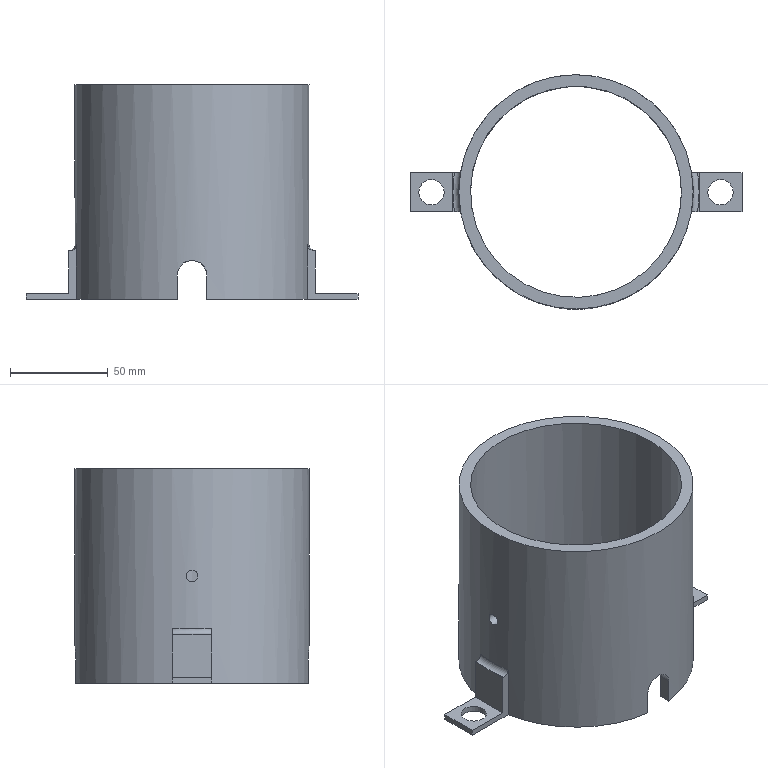Part | NX | features solid 2 | 1 solid | 30 faces | box 170 x 120 x 110 mm | volume 238085 mm3 | plane 21 | cylinder 7 | torus 2 | commonest cylinder face diameters 13 x2 15 x2 6 x1 108 x1 120 x1
STEP:
#1=CARTESIAN_POINT('',(1017.5,-595.,-130.));
#2=VERTEX_POINT('',#1);
#3=CARTESIAN_POINT('',(1011.,-595.,-130.));
#4=DIRECTION('',(0.,0.,1.));
#5=DIRECTION('',(1.,0.,0.));
#6=AXIS2_PLACEMENT_3D('',#3,#4,#5);
#7=CIRCLE('',#6,6.5);
#8=EDGE_CURVE('',#2,#2,#7,.T.);
#9=ORIENTED_EDGE('',*,*,#8,.T.);
#10=EDGE_LOOP('',(#9));
#11=FACE_BOUND('',#10,.T.);
#12=CARTESIAN_POINT('',(1077.5,-535.471,-130.));
#13=VERTEX_POINT('',#12);
#14=CARTESIAN_POINT('',(1025.839,-585.,-130.));
#15=VERTEX_POINT('',#14);
#16=CARTESIAN_POINT('',(1085.,-595.,-130.));
#17=DIRECTION('',(0.,0.,1.));
#18=DIRECTION('',(1.,0.,0.));
#19=AXIS2_PLACEMENT_3D('',#16,#17,#18);
#20=CIRCLE('',#19,60.);
#21=EDGE_CURVE('',#13,#15,#20,.T.);
#22=ORIENTED_EDGE('',*,*,#21,.F.);
#23=CARTESIAN_POINT('',(1077.5,-541.523,-130.));
#24=VERTEX_POINT('',#23);
#25=CARTESIAN_POINT('',(1077.5,-595.,-130.));
#26=DIRECTION('',(0.,-1.,0.));
#27=VECTOR('',#26,1000.);
#28=LINE('',#25,#27);
#29=EDGE_CURVE('',#13,#24,#28,.T.);
#30=ORIENTED_EDGE('',*,*,#29,.T.);
#31=CARTESIAN_POINT('',(1077.5,-648.477,-130.));
#32=VERTEX_POINT('',#31);
#33=CARTESIAN_POINT('',(1085.,-595.,-130.));
#34=DIRECTION('',(0.,0.,1.));
#35=DIRECTION('',(1.,0.,0.));
#36=AXIS2_PLACEMENT_3D('',#33,#34,#35);
#37=CIRCLE('',#36,54.);
#38=EDGE_CURVE('',#24,#32,#37,.T.);
#39=ORIENTED_EDGE('',*,*,#38,.T.);
#40=CARTESIAN_POINT('',(1077.5,-654.529,-130.));
#41=VERTEX_POINT('',#40);
#42=CARTESIAN_POINT('',(1077.5,-595.,-130.));
#43=DIRECTION('',(0.,-1.,0.));
#44=VECTOR('',#43,1000.);
#45=LINE('',#42,#44);
#46=EDGE_CURVE('',#32,#41,#45,.T.);
#47=ORIENTED_EDGE('',*,*,#46,.T.);
#48=CARTESIAN_POINT('',(1025.839,-605.,-130.));
#49=VERTEX_POINT('',#48);
#50=CARTESIAN_POINT('',(1085.,-595.,-130.));
#51=DIRECTION('',(0.,0.,1.));
#52=DIRECTION('',(1.,0.,0.));
#53=AXIS2_PLACEMENT_3D('',#50,#51,#52);
#54=CIRCLE('',#53,60.);
#55=EDGE_CURVE('',#49,#41,#54,.T.);
#56=ORIENTED_EDGE('',*,*,#55,.F.);
#57=CARTESIAN_POINT('',(1000.,-605.,-130.));
#58=VERTEX_POINT('',#57);
#59=CARTESIAN_POINT('',(1022.,-605.,-130.));
#60=DIRECTION('',(1.,0.,0.));
#61=VECTOR('',#60,1000.);
#62=LINE('',#59,#61);
#63=EDGE_CURVE('',#58,#49,#62,.T.);
#64=ORIENTED_EDGE('',*,*,#63,.F.);
#65=CARTESIAN_POINT('',(1000.,-585.,-130.));
#66=VERTEX_POINT('',#65);
#67=CARTESIAN_POINT('',(1000.,-605.,-130.));
#68=DIRECTION('',(0.,1.,0.));
#69=VECTOR('',#68,1000.);
#70=LINE('',#67,#69);
#71=EDGE_CURVE('',#58,#66,#70,.T.);
#72=ORIENTED_EDGE('',*,*,#71,.T.);
#73=CARTESIAN_POINT('',(1031.,-585.,-130.));
#74=DIRECTION('',(-1.,0.,0.));
#75=VECTOR('',#74,1000.);
#76=LINE('',#73,#75);
#77=EDGE_CURVE('',#15,#66,#76,.T.);
#78=ORIENTED_EDGE('',*,*,#77,.F.);
#79=EDGE_LOOP('',(#22,#30,#39,#47,#56,#64,#72,#78));
#80=FACE_BOUND('',#79,.T.);
#81=CARTESIAN_POINT('',(1085.,-595.,-130.));
#82=DIRECTION('',(0.,0.,1.));
#83=DIRECTION('',(1.,0.,0.));
#84=AXIS2_PLACEMENT_3D('',#81,#82,#83);
#85=PLANE('',#84);
#86=ADVANCED_FACE('',(#11,#80),#85,.F.);
#87=CARTESIAN_POINT('',(1148.,-585.,-105.));
#88=VERTEX_POINT('',#87);
#89=CARTESIAN_POINT('',(1147.201,-585.,-105.));
#90=VERTEX_POINT('',#89);
#91=CARTESIAN_POINT('',(1148.,-585.,-105.));
#92=DIRECTION('',(-1.,0.,0.));
#93=VECTOR('',#92,1000.);
#94=LINE('',#91,#93);
#95=EDGE_CURVE('',#88,#90,#94,.T.);
#96=ORIENTED_EDGE('',*,*,#95,.T.);
#97=CARTESIAN_POINT('',(1148.,-595.,-105.));
#98=VERTEX_POINT('',#97);
#99=CARTESIAN_POINT('',(1085.,-595.,-105.));
#100=DIRECTION('',(0.,0.,1.));
#101=DIRECTION('',(1.,0.,0.));
#102=AXIS2_PLACEMENT_3D('',#99,#100,#101);
#103=CIRCLE('',#102,63.);
#104=EDGE_CURVE('',#90,#98,#103,.F.);
#105=ORIENTED_EDGE('',*,*,#104,.T.);
#106=CARTESIAN_POINT('',(1148.,-605.,-105.));
#107=DIRECTION('',(0.,1.,0.));
#108=VECTOR('',#107,1000.);
#109=LINE('',#106,#108);
#110=EDGE_CURVE('',#98,#88,#109,.T.);
#111=ORIENTED_EDGE('',*,*,#110,.T.);
#112=EDGE_LOOP('',(#96,#105,#111));
#113=FACE_BOUND('',#112,.T.);
#114=CARTESIAN_POINT('',(1139.,-585.,-105.));
#115=DIRECTION('',(0.,0.,1.));
#116=DIRECTION('',(1.,0.,0.));
#117=AXIS2_PLACEMENT_3D('',#114,#115,#116);
#118=PLANE('',#117);
#119=ADVANCED_FACE('',(#113),#118,.T.);
#120=CARTESIAN_POINT('',(1022.,-605.,-105.));
#121=VERTEX_POINT('',#120);
#122=CARTESIAN_POINT('',(1022.799,-605.,-105.));
#123=VERTEX_POINT('',#122);
#124=CARTESIAN_POINT('',(1022.,-605.,-105.));
#125=DIRECTION('',(1.,0.,0.));
#126=VECTOR('',#125,1000.);
#127=LINE('',#124,#126);
#128=EDGE_CURVE('',#121,#123,#127,.T.);
#129=ORIENTED_EDGE('',*,*,#128,.T.);
#130=CARTESIAN_POINT('',(1022.,-595.,-105.));
#131=VERTEX_POINT('',#130);
#132=CARTESIAN_POINT('',(1085.,-595.,-105.));
#133=DIRECTION('',(0.,0.,-1.));
#134=DIRECTION('',(-1.,0.,0.));
#135=AXIS2_PLACEMENT_3D('',#132,#133,#134);
#136=CIRCLE('',#135,63.);
#137=EDGE_CURVE('',#123,#131,#136,.T.);
#138=ORIENTED_EDGE('',*,*,#137,.T.);
#139=CARTESIAN_POINT('',(1022.,-585.,-105.));
#140=DIRECTION('',(0.,-1.,0.));
#141=VECTOR('',#140,1000.);
#142=LINE('',#139,#141);
#143=EDGE_CURVE('',#131,#121,#142,.T.);
#144=ORIENTED_EDGE('',*,*,#143,.T.);
#145=EDGE_LOOP('',(#129,#138,#144));
#146=FACE_BOUND('',#145,.T.);
#147=CARTESIAN_POINT('',(1022.,-585.,-105.));
#148=DIRECTION('',(0.,0.,-1.));
#149=DIRECTION('',(-1.,0.,0.));
#150=AXIS2_PLACEMENT_3D('',#147,#148,#149);
#151=PLANE('',#150);
#152=ADVANCED_FACE('',(#146),#151,.F.);
#153=CARTESIAN_POINT('',(1025.,-595.,-72.));
#154=VERTEX_POINT('',#153);
#155=CARTESIAN_POINT('',(1025.038,-592.647,-72.651));
#156=CARTESIAN_POINT('',(1024.981,-595.001,-71.675));
#157=CARTESIAN_POINT('',(1025.038,-597.351,-72.65));
#158=CARTESIAN_POINT('',(1025.094,-598.324,-74.998));
#159=CARTESIAN_POINT('',(1025.038,-597.352,-77.35));
#160=CARTESIAN_POINT('',(1024.981,-595.,-78.324));
#161=CARTESIAN_POINT('',(1025.037,-592.652,-77.353));
#162=CARTESIAN_POINT('',(1025.094,-591.675,-75.003));
#163=CARTESIAN_POINT('',(1025.038,-592.647,-72.651));
#164=CARTESIAN_POINT('',(1024.981,-595.001,-71.675));
#165=CARTESIAN_POINT('',(1025.038,-597.351,-72.65));
#166=B_SPLINE_CURVE_WITH_KNOTS('',3,(#155,#156,#157,#158,#159,#160,#161,#162,#163,#164,#165),.UNSPECIFIED.,.T.,.F.,(1,1,1,1,1,1,1,1,1,1,1,1,1,1,1),(-0.007035,-0.00469,-0.002345,0.,0.002345,0.00469,0.007035,0.00938,0.01172,0.01407,0.01641,0.01876,0.0211,0.02345,0.02579),.UNSPECIFIED.);
#167=EDGE_CURVE('',#154,#154,#166,.T.);
#168=ORIENTED_EDGE('',*,*,#167,.T.);
#169=EDGE_LOOP('',(#168));
#170=FACE_BOUND('',#169,.T.);
#171=CARTESIAN_POINT('',(1145.,-595.,-20.));
#172=VERTEX_POINT('',#171);
#173=CARTESIAN_POINT('',(1085.,-595.,-20.));
#174=DIRECTION('',(0.,0.,1.));
#175=DIRECTION('',(1.,0.,0.));
#176=AXIS2_PLACEMENT_3D('',#173,#174,#175);
#177=CIRCLE('',#176,60.);
#178=EDGE_CURVE('',#172,#172,#177,.T.);
#179=ORIENTED_EDGE('',*,*,#178,.F.);
#180=EDGE_LOOP('',(#179));
#181=FACE_BOUND('',#180,.T.);
#182=CARTESIAN_POINT('',(1092.5,-535.471,-117.5));
#183=VERTEX_POINT('',#182);
#184=CARTESIAN_POINT('',(1077.5,-535.471,-117.5));
#185=VERTEX_POINT('',#184);
#186=CARTESIAN_POINT('',(1092.5,-535.471,-117.5));
#187=CARTESIAN_POINT('',(1092.5,-535.471,-115.516));
#188=CARTESIAN_POINT('',(1090.875,-535.234,-111.635));
#189=CARTESIAN_POINT('',(1085.008,-534.883,-109.184));
#190=CARTESIAN_POINT('',(1079.127,-535.234,-111.629));
#191=CARTESIAN_POINT('',(1077.5,-535.471,-115.516));
#192=CARTESIAN_POINT('',(1077.5,-535.471,-117.5));
#193=B_SPLINE_CURVE_WITH_KNOTS('',3,(#186,#187,#188,#189,#190,#191,#192),.UNSPECIFIED.,.F.,.F.,(4,1,1,1,4),(0.,0.005866,0.01173,0.0176,0.02347),.UNSPECIFIED.);
#194=EDGE_CURVE('',#183,#185,#193,.T.);
#195=ORIENTED_EDGE('',*,*,#194,.T.);
#196=CARTESIAN_POINT('',(1077.5,-535.471,-20.));
#197=DIRECTION('',(0.,0.,-1.));
#198=VECTOR('',#197,1000.);
#199=LINE('',#196,#198);
#200=EDGE_CURVE('',#185,#13,#199,.T.);
#201=ORIENTED_EDGE('',*,*,#200,.T.);
#202=ORIENTED_EDGE('',*,*,#21,.T.);
#203=CARTESIAN_POINT('',(1025.839,-585.,-102.));
#204=VERTEX_POINT('',#203);
#205=CARTESIAN_POINT('',(1025.839,-585.,-20.));
#206=DIRECTION('',(0.,0.,-1.));
#207=VECTOR('',#206,1000.);
#208=LINE('',#205,#207);
#209=EDGE_CURVE('',#204,#15,#208,.T.);
#210=ORIENTED_EDGE('',*,*,#209,.F.);
#211=CARTESIAN_POINT('',(1025.839,-605.,-102.));
#212=VERTEX_POINT('',#211);
#213=CARTESIAN_POINT('',(1085.,-595.,-102.));
#214=DIRECTION('',(0.,0.,-1.));
#215=DIRECTION('',(-1.,0.,0.));
#216=AXIS2_PLACEMENT_3D('',#213,#214,#215);
#217=CIRCLE('',#216,60.);
#218=EDGE_CURVE('',#204,#212,#217,.F.);
#219=ORIENTED_EDGE('',*,*,#218,.T.);
#220=CARTESIAN_POINT('',(1025.839,-605.,-20.));
#221=DIRECTION('',(0.,0.,-1.));
#222=VECTOR('',#221,1000.);
#223=LINE('',#220,#222);
#224=EDGE_CURVE('',#49,#212,#223,.F.);
#225=ORIENTED_EDGE('',*,*,#224,.F.);
#226=ORIENTED_EDGE('',*,*,#55,.T.);
#227=CARTESIAN_POINT('',(1077.5,-654.529,-117.5));
#228=VERTEX_POINT('',#227);
#229=CARTESIAN_POINT('',(1077.5,-654.529,-20.));
#230=DIRECTION('',(0.,0.,-1.));
#231=VECTOR('',#230,1000.);
#232=LINE('',#229,#231);
#233=EDGE_CURVE('',#41,#228,#232,.F.);
#234=ORIENTED_EDGE('',*,*,#233,.T.);
#235=CARTESIAN_POINT('',(1092.5,-654.529,-117.5));
#236=VERTEX_POINT('',#235);
#237=CARTESIAN_POINT('',(1077.5,-654.529,-117.5));
#238=CARTESIAN_POINT('',(1077.5,-654.529,-115.516));
#239=CARTESIAN_POINT('',(1079.125,-654.766,-111.635));
#240=CARTESIAN_POINT('',(1084.992,-655.117,-109.184));
#241=CARTESIAN_POINT('',(1090.873,-654.766,-111.629));
#242=CARTESIAN_POINT('',(1092.5,-654.529,-115.516));
#243=CARTESIAN_POINT('',(1092.5,-654.529,-117.5));
#244=B_SPLINE_CURVE_WITH_KNOTS('',3,(#237,#238,#239,#240,#241,#242,#243),.UNSPECIFIED.,.F.,.F.,(4,1,1,1,4),(0.,0.005866,0.01173,0.0176,0.02347),.UNSPECIFIED.);
#245=EDGE_CURVE('',#228,#236,#244,.T.);
#246=ORIENTED_EDGE('',*,*,#245,.T.);
#247=CARTESIAN_POINT('',(1092.5,-654.529,-130.));
#248=VERTEX_POINT('',#247);
#249=CARTESIAN_POINT('',(1092.5,-654.529,-20.));
#250=DIRECTION('',(0.,0.,-1.));
#251=VECTOR('',#250,1000.);
#252=LINE('',#249,#251);
#253=EDGE_CURVE('',#236,#248,#252,.T.);
#254=ORIENTED_EDGE('',*,*,#253,.T.);
#255=CARTESIAN_POINT('',(1144.161,-605.,-130.));
#256=VERTEX_POINT('',#255);
#257=CARTESIAN_POINT('',(1085.,-595.,-130.));
#258=DIRECTION('',(0.,0.,1.));
#259=DIRECTION('',(1.,0.,0.));
#260=AXIS2_PLACEMENT_3D('',#257,#258,#259);
#261=CIRCLE('',#260,60.);
#262=EDGE_CURVE('',#248,#256,#261,.T.);
#263=ORIENTED_EDGE('',*,*,#262,.T.);
#264=CARTESIAN_POINT('',(1144.161,-605.,-102.));
#265=VERTEX_POINT('',#264);
#266=CARTESIAN_POINT('',(1144.161,-605.,-20.));
#267=DIRECTION('',(0.,0.,-1.));
#268=VECTOR('',#267,1000.);
#269=LINE('',#266,#268);
#270=EDGE_CURVE('',#265,#256,#269,.T.);
#271=ORIENTED_EDGE('',*,*,#270,.F.);
#272=CARTESIAN_POINT('',(1144.161,-585.,-102.));
#273=VERTEX_POINT('',#272);
#274=CARTESIAN_POINT('',(1085.,-595.,-102.));
#275=DIRECTION('',(0.,0.,1.));
#276=DIRECTION('',(1.,0.,0.));
#277=AXIS2_PLACEMENT_3D('',#274,#275,#276);
#278=CIRCLE('',#277,60.);
#279=EDGE_CURVE('',#265,#273,#278,.T.);
#280=ORIENTED_EDGE('',*,*,#279,.T.);
#281=CARTESIAN_POINT('',(1144.161,-585.,-130.));
#282=VERTEX_POINT('',#281);
#283=CARTESIAN_POINT('',(1144.161,-585.,-20.));
#284=DIRECTION('',(0.,0.,-1.));
#285=VECTOR('',#284,1000.);
#286=LINE('',#283,#285);
#287=EDGE_CURVE('',#282,#273,#286,.F.);
#288=ORIENTED_EDGE('',*,*,#287,.F.);
#289=CARTESIAN_POINT('',(1092.5,-535.471,-130.));
#290=VERTEX_POINT('',#289);
#291=CARTESIAN_POINT('',(1085.,-595.,-130.));
#292=DIRECTION('',(0.,0.,1.));
#293=DIRECTION('',(1.,0.,0.));
#294=AXIS2_PLACEMENT_3D('',#291,#292,#293);
#295=CIRCLE('',#294,60.);
#296=EDGE_CURVE('',#282,#290,#295,.T.);
#297=ORIENTED_EDGE('',*,*,#296,.T.);
#298=CARTESIAN_POINT('',(1092.5,-535.471,-20.));
#299=DIRECTION('',(0.,0.,-1.));
#300=VECTOR('',#299,1000.);
#301=LINE('',#298,#300);
#302=EDGE_CURVE('',#290,#183,#301,.F.);
#303=ORIENTED_EDGE('',*,*,#302,.T.);
#304=EDGE_LOOP('',(#195,#201,#202,#210,#219,#225,#226,#234,#246,#254,#263,#271,#280,#288,#297,#303));
#305=FACE_BOUND('',#304,.T.);
#306=CARTESIAN_POINT('',(1085.,-595.,-20.));
#307=DIRECTION('',(0.,0.,-1.));
#308=DIRECTION('',(-1.,0.,0.));
#309=AXIS2_PLACEMENT_3D('',#306,#307,#308);
#310=CYLINDRICAL_SURFACE('',#309,60.);
#311=ADVANCED_FACE('',(#170,#181,#305),#310,.T.);
#312=CARTESIAN_POINT('',(1077.5,-541.523,-117.5));
#313=VERTEX_POINT('',#312);
#314=CARTESIAN_POINT('',(1077.5,-541.523,-20.));
#315=DIRECTION('',(0.,0.,-1.));
#316=VECTOR('',#315,1000.);
#317=LINE('',#314,#316);
#318=EDGE_CURVE('',#313,#24,#317,.T.);
#319=ORIENTED_EDGE('',*,*,#318,.F.);
#320=CARTESIAN_POINT('',(1092.5,-541.523,-117.5));
#321=VERTEX_POINT('',#320);
#322=CARTESIAN_POINT('',(1092.5,-541.523,-117.5));
#323=CARTESIAN_POINT('',(1092.5,-541.523,-115.516));
#324=CARTESIAN_POINT('',(1090.875,-541.26,-111.635));
#325=CARTESIAN_POINT('',(1085.008,-540.87,-109.184));
#326=CARTESIAN_POINT('',(1079.126,-541.26,-111.629));
#327=CARTESIAN_POINT('',(1077.5,-541.523,-115.516));
#328=CARTESIAN_POINT('',(1077.5,-541.523,-117.5));
#329=B_SPLINE_CURVE_WITH_KNOTS('',3,(#322,#323,#324,#325,#326,#327,#328),.UNSPECIFIED.,.F.,.F.,(4,1,1,1,4),(0.,0.005868,0.01174,0.0176,0.02347),.UNSPECIFIED.);
#330=EDGE_CURVE('',#321,#313,#329,.T.);
#331=ORIENTED_EDGE('',*,*,#330,.F.);
#332=CARTESIAN_POINT('',(1092.5,-541.523,-130.));
#333=VERTEX_POINT('',#332);
#334=CARTESIAN_POINT('',(1092.5,-541.523,-20.));
#335=DIRECTION('',(0.,0.,-1.));
#336=VECTOR('',#335,1000.);
#337=LINE('',#334,#336);
#338=EDGE_CURVE('',#333,#321,#337,.F.);
#339=ORIENTED_EDGE('',*,*,#338,.F.);
#340=CARTESIAN_POINT('',(1092.5,-648.477,-130.));
#341=VERTEX_POINT('',#340);
#342=CARTESIAN_POINT('',(1085.,-595.,-130.));
#343=DIRECTION('',(0.,0.,1.));
#344=DIRECTION('',(1.,0.,0.));
#345=AXIS2_PLACEMENT_3D('',#342,#343,#344);
#346=CIRCLE('',#345,54.);
#347=EDGE_CURVE('',#341,#333,#346,.T.);
#348=ORIENTED_EDGE('',*,*,#347,.F.);
#349=CARTESIAN_POINT('',(1092.5,-648.477,-117.5));
#350=VERTEX_POINT('',#349);
#351=CARTESIAN_POINT('',(1092.5,-648.477,-20.));
#352=DIRECTION('',(0.,0.,-1.));
#353=VECTOR('',#352,1000.);
#354=LINE('',#351,#353);
#355=EDGE_CURVE('',#350,#341,#354,.T.);
#356=ORIENTED_EDGE('',*,*,#355,.F.);
#357=CARTESIAN_POINT('',(1077.5,-648.477,-117.5));
#358=VERTEX_POINT('',#357);
#359=CARTESIAN_POINT('',(1077.5,-648.477,-117.5));
#360=CARTESIAN_POINT('',(1077.5,-648.477,-115.516));
#361=CARTESIAN_POINT('',(1079.125,-648.74,-111.635));
#362=CARTESIAN_POINT('',(1084.992,-649.13,-109.184));
#363=CARTESIAN_POINT('',(1090.874,-648.74,-111.629));
#364=CARTESIAN_POINT('',(1092.5,-648.477,-115.516));
#365=CARTESIAN_POINT('',(1092.5,-648.477,-117.5));
#366=B_SPLINE_CURVE_WITH_KNOTS('',3,(#359,#360,#361,#362,#363,#364,#365),.UNSPECIFIED.,.F.,.F.,(4,1,1,1,4),(0.,0.005868,0.01174,0.0176,0.02347),.UNSPECIFIED.);
#367=EDGE_CURVE('',#358,#350,#366,.T.);
#368=ORIENTED_EDGE('',*,*,#367,.F.);
#369=CARTESIAN_POINT('',(1077.5,-648.477,-20.));
#370=DIRECTION('',(0.,0.,-1.));
#371=VECTOR('',#370,1000.);
#372=LINE('',#369,#371);
#373=EDGE_CURVE('',#32,#358,#372,.F.);
#374=ORIENTED_EDGE('',*,*,#373,.F.);
#375=ORIENTED_EDGE('',*,*,#38,.F.);
#376=EDGE_LOOP('',(#319,#331,#339,#348,#356,#368,#374,#375));
#377=FACE_BOUND('',#376,.T.);
#378=CARTESIAN_POINT('',(1031.,-595.,-72.));
#379=VERTEX_POINT('',#378);
#380=CARTESIAN_POINT('',(1031.042,-592.647,-72.651));
#381=CARTESIAN_POINT('',(1030.979,-595.001,-71.675));
#382=CARTESIAN_POINT('',(1031.042,-597.351,-72.65));
#383=CARTESIAN_POINT('',(1031.104,-598.324,-74.998));
#384=CARTESIAN_POINT('',(1031.042,-597.352,-77.35));
#385=CARTESIAN_POINT('',(1030.979,-595.,-78.324));
#386=CARTESIAN_POINT('',(1031.042,-592.652,-77.353));
#387=CARTESIAN_POINT('',(1031.104,-591.675,-75.003));
#388=CARTESIAN_POINT('',(1031.042,-592.647,-72.651));
#389=CARTESIAN_POINT('',(1030.979,-595.001,-71.675));
#390=CARTESIAN_POINT('',(1031.042,-597.351,-72.65));
#391=B_SPLINE_CURVE_WITH_KNOTS('',3,(#380,#381,#382,#383,#384,#385,#386,#387,#388,#389,#390),.UNSPECIFIED.,.T.,.F.,(1,1,1,1,1,1,1,1,1,1,1,1,1,1,1),(-0.007035,-0.00469,-0.002345,0.,0.002345,0.00469,0.007035,0.00938,0.01173,0.01407,0.01642,0.01876,0.02111,0.02345,0.0258),.UNSPECIFIED.);
#392=EDGE_CURVE('',#379,#379,#391,.T.);
#393=ORIENTED_EDGE('',*,*,#392,.F.);
#394=EDGE_LOOP('',(#393));
#395=FACE_BOUND('',#394,.T.);
#396=CARTESIAN_POINT('',(1139.,-595.,-20.));
#397=VERTEX_POINT('',#396);
#398=CARTESIAN_POINT('',(1085.,-595.,-20.));
#399=DIRECTION('',(0.,0.,1.));
#400=DIRECTION('',(1.,0.,0.));
#401=AXIS2_PLACEMENT_3D('',#398,#399,#400);
#402=CIRCLE('',#401,54.);
#403=EDGE_CURVE('',#397,#397,#402,.T.);
#404=ORIENTED_EDGE('',*,*,#403,.T.);
#405=EDGE_LOOP('',(#404));
#406=FACE_BOUND('',#405,.T.);
#407=CARTESIAN_POINT('',(1085.,-595.,-20.));
#408=DIRECTION('',(0.,0.,-1.));
#409=DIRECTION('',(-1.,0.,0.));
#410=AXIS2_PLACEMENT_3D('',#407,#408,#409);
#411=CYLINDRICAL_SURFACE('',#410,54.);
#412=ADVANCED_FACE('',(#377,#395,#406),#411,.F.);
#413=ORIENTED_EDGE('',*,*,#403,.F.);
#414=EDGE_LOOP('',(#413));
#415=FACE_BOUND('',#414,.T.);
#416=ORIENTED_EDGE('',*,*,#178,.T.);
#417=EDGE_LOOP('',(#416));
#418=FACE_BOUND('',#417,.T.);
#419=CARTESIAN_POINT('',(1085.,-595.,-20.));
#420=DIRECTION('',(0.,0.,1.));
#421=DIRECTION('',(1.,0.,0.));
#422=AXIS2_PLACEMENT_3D('',#419,#420,#421);
#423=PLANE('',#422);
#424=ADVANCED_FACE('',(#415,#418),#423,.T.);
#425=ORIENTED_EDGE('',*,*,#347,.T.);
#426=CARTESIAN_POINT('',(1092.5,-595.,-130.));
#427=DIRECTION('',(0.,1.,0.));
#428=VECTOR('',#427,1000.);
#429=LINE('',#426,#428);
#430=EDGE_CURVE('',#333,#290,#429,.T.);
#431=ORIENTED_EDGE('',*,*,#430,.T.);
#432=ORIENTED_EDGE('',*,*,#296,.F.);
#433=CARTESIAN_POINT('',(1170.,-585.,-130.));
#434=VERTEX_POINT('',#433);
#435=CARTESIAN_POINT('',(1148.,-585.,-130.));
#436=DIRECTION('',(-1.,0.,0.));
#437=VECTOR('',#436,1000.);
#438=LINE('',#435,#437);
#439=EDGE_CURVE('',#434,#282,#438,.T.);
#440=ORIENTED_EDGE('',*,*,#439,.F.);
#441=CARTESIAN_POINT('',(1170.,-605.,-130.));
#442=VERTEX_POINT('',#441);
#443=CARTESIAN_POINT('',(1170.,-585.,-130.));
#444=DIRECTION('',(0.,-1.,0.));
#445=VECTOR('',#444,1000.);
#446=LINE('',#443,#445);
#447=EDGE_CURVE('',#434,#442,#446,.T.);
#448=ORIENTED_EDGE('',*,*,#447,.T.);
#449=CARTESIAN_POINT('',(1139.,-605.,-130.));
#450=DIRECTION('',(1.,0.,0.));
#451=VECTOR('',#450,1000.);
#452=LINE('',#449,#451);
#453=EDGE_CURVE('',#256,#442,#452,.T.);
#454=ORIENTED_EDGE('',*,*,#453,.F.);
#455=ORIENTED_EDGE('',*,*,#262,.F.);
#456=CARTESIAN_POINT('',(1092.5,-595.,-130.));
#457=DIRECTION('',(0.,1.,0.));
#458=VECTOR('',#457,1000.);
#459=LINE('',#456,#458);
#460=EDGE_CURVE('',#248,#341,#459,.T.);
#461=ORIENTED_EDGE('',*,*,#460,.T.);
#462=EDGE_LOOP('',(#425,#431,#432,#440,#448,#454,#455,#461));
#463=FACE_BOUND('',#462,.T.);
#464=CARTESIAN_POINT('',(1165.5,-595.,-130.));
#465=VERTEX_POINT('',#464);
#466=CARTESIAN_POINT('',(1159.,-595.,-130.));
#467=DIRECTION('',(0.,0.,1.));
#468=DIRECTION('',(1.,0.,0.));
#469=AXIS2_PLACEMENT_3D('',#466,#467,#468);
#470=CIRCLE('',#469,6.5);
#471=EDGE_CURVE('',#465,#465,#470,.T.);
#472=ORIENTED_EDGE('',*,*,#471,.T.);
#473=EDGE_LOOP('',(#472));
#474=FACE_BOUND('',#473,.T.);
#475=CARTESIAN_POINT('',(1085.,-595.,-130.));
#476=DIRECTION('',(0.,0.,1.));
#477=DIRECTION('',(1.,0.,0.));
#478=AXIS2_PLACEMENT_3D('',#475,#476,#477);
#479=PLANE('',#478);
#480=ADVANCED_FACE('',(#463,#474),#479,.F.);
#481=CARTESIAN_POINT('',(1022.,-585.,-105.));
#482=VERTEX_POINT('',#481);
#483=CARTESIAN_POINT('',(1022.,-585.,-105.));
#484=DIRECTION('',(0.,-1.,0.));
#485=VECTOR('',#484,1000.);
#486=LINE('',#483,#485);
#487=EDGE_CURVE('',#482,#131,#486,.T.);
#488=ORIENTED_EDGE('',*,*,#487,.T.);
#489=CARTESIAN_POINT('',(1022.799,-585.,-105.));
#490=VERTEX_POINT('',#489);
#491=CARTESIAN_POINT('',(1085.,-595.,-105.));
#492=DIRECTION('',(0.,0.,-1.));
#493=DIRECTION('',(-1.,0.,0.));
#494=AXIS2_PLACEMENT_3D('',#491,#492,#493);
#495=CIRCLE('',#494,63.);
#496=EDGE_CURVE('',#131,#490,#495,.T.);
#497=ORIENTED_EDGE('',*,*,#496,.T.);
#498=CARTESIAN_POINT('',(1031.,-585.,-105.));
#499=DIRECTION('',(-1.,0.,0.));
#500=VECTOR('',#499,1000.);
#501=LINE('',#498,#500);
#502=EDGE_CURVE('',#490,#482,#501,.T.);
#503=ORIENTED_EDGE('',*,*,#502,.T.);
#504=EDGE_LOOP('',(#488,#497,#503));
#505=FACE_BOUND('',#504,.T.);
#506=CARTESIAN_POINT('',(1022.,-585.,-105.));
#507=DIRECTION('',(0.,0.,-1.));
#508=DIRECTION('',(-1.,0.,0.));
#509=AXIS2_PLACEMENT_3D('',#506,#507,#508);
#510=PLANE('',#509);
#511=ADVANCED_FACE('',(#505),#510,.F.);
#512=ORIENTED_EDGE('',*,*,#63,.T.);
#513=ORIENTED_EDGE('',*,*,#224,.T.);
#514=CARTESIAN_POINT('',(1025.839,-605.,-102.));
#515=CARTESIAN_POINT('',(1025.839,-605.,-102.798));
#516=CARTESIAN_POINT('',(1025.166,-605.,-104.356));
#517=CARTESIAN_POINT('',(1023.596,-605.,-105.));
#518=CARTESIAN_POINT('',(1022.799,-605.,-105.));
#519=B_SPLINE_CURVE_WITH_KNOTS('',3,(#514,#515,#516,#517,#518),.UNSPECIFIED.,.F.,.F.,(4,1,4),(0.,0.002359,0.004718),.UNSPECIFIED.);
#520=EDGE_CURVE('',#212,#123,#519,.T.);
#521=ORIENTED_EDGE('',*,*,#520,.T.);
#522=ORIENTED_EDGE('',*,*,#128,.F.);
#523=CARTESIAN_POINT('',(1022.,-605.,-127.));
#524=VERTEX_POINT('',#523);
#525=CARTESIAN_POINT('',(1022.,-605.,-105.));
#526=DIRECTION('',(0.,0.,-1.));
#527=VECTOR('',#526,1000.);
#528=LINE('',#525,#527);
#529=EDGE_CURVE('',#121,#524,#528,.T.);
#530=ORIENTED_EDGE('',*,*,#529,.T.);
#531=CARTESIAN_POINT('',(1000.,-605.,-127.));
#532=VERTEX_POINT('',#531);
#533=CARTESIAN_POINT('',(1022.,-605.,-127.));
#534=DIRECTION('',(-1.,0.,0.));
#535=VECTOR('',#534,1000.);
#536=LINE('',#533,#535);
#537=EDGE_CURVE('',#524,#532,#536,.T.);
#538=ORIENTED_EDGE('',*,*,#537,.T.);
#539=CARTESIAN_POINT('',(1000.,-605.,-127.));
#540=DIRECTION('',(0.,0.,-1.));
#541=VECTOR('',#540,1000.);
#542=LINE('',#539,#541);
#543=EDGE_CURVE('',#532,#58,#542,.T.);
#544=ORIENTED_EDGE('',*,*,#543,.T.);
#545=EDGE_LOOP('',(#512,#513,#521,#522,#530,#538,#544));
#546=FACE_BOUND('',#545,.T.);
#547=CARTESIAN_POINT('',(1022.,-605.,-105.));
#548=DIRECTION('',(0.,1.,0.));
#549=DIRECTION('',(-1.,0.,0.));
#550=AXIS2_PLACEMENT_3D('',#547,#548,#549);
#551=PLANE('',#550);
#552=ADVANCED_FACE('',(#546),#551,.F.);
#553=ORIENTED_EDGE('',*,*,#502,.F.);
#554=CARTESIAN_POINT('',(1022.799,-585.,-105.));
#555=CARTESIAN_POINT('',(1023.596,-585.,-105.));
#556=CARTESIAN_POINT('',(1025.163,-585.,-104.359));
#557=CARTESIAN_POINT('',(1025.839,-585.,-102.798));
#558=CARTESIAN_POINT('',(1025.839,-585.,-102.));
#559=B_SPLINE_CURVE_WITH_KNOTS('',3,(#554,#555,#556,#557,#558),.UNSPECIFIED.,.F.,.F.,(4,1,4),(0.,0.002359,0.004718),.UNSPECIFIED.);
#560=EDGE_CURVE('',#490,#204,#559,.T.);
#561=ORIENTED_EDGE('',*,*,#560,.T.);
#562=ORIENTED_EDGE('',*,*,#209,.T.);
#563=ORIENTED_EDGE('',*,*,#77,.T.);
#564=CARTESIAN_POINT('',(1000.,-585.,-127.));
#565=VERTEX_POINT('',#564);
#566=CARTESIAN_POINT('',(1000.,-585.,-127.));
#567=DIRECTION('',(0.,0.,-1.));
#568=VECTOR('',#567,1000.);
#569=LINE('',#566,#568);
#570=EDGE_CURVE('',#565,#66,#569,.T.);
#571=ORIENTED_EDGE('',*,*,#570,.F.);
#572=CARTESIAN_POINT('',(1022.,-585.,-127.));
#573=VERTEX_POINT('',#572);
#574=CARTESIAN_POINT('',(1000.,-585.,-127.));
#575=DIRECTION('',(1.,0.,0.));
#576=VECTOR('',#575,1000.);
#577=LINE('',#574,#576);
#578=EDGE_CURVE('',#565,#573,#577,.T.);
#579=ORIENTED_EDGE('',*,*,#578,.T.);
#580=CARTESIAN_POINT('',(1022.,-585.,-105.));
#581=DIRECTION('',(0.,0.,-1.));
#582=VECTOR('',#581,1000.);
#583=LINE('',#580,#582);
#584=EDGE_CURVE('',#482,#573,#583,.T.);
#585=ORIENTED_EDGE('',*,*,#584,.F.);
#586=EDGE_LOOP('',(#553,#561,#562,#563,#571,#579,#585));
#587=FACE_BOUND('',#586,.T.);
#588=CARTESIAN_POINT('',(1031.,-585.,-105.));
#589=DIRECTION('',(0.,-1.,0.));
#590=DIRECTION('',(0.,0.,-1.));
#591=AXIS2_PLACEMENT_3D('',#588,#589,#590);
#592=PLANE('',#591);
#593=ADVANCED_FACE('',(#587),#592,.F.);
#594=ORIENTED_EDGE('',*,*,#584,.T.);
#595=CARTESIAN_POINT('',(1022.,-585.,-127.));
#596=DIRECTION('',(0.,-1.,0.));
#597=VECTOR('',#596,1000.);
#598=LINE('',#595,#597);
#599=EDGE_CURVE('',#573,#524,#598,.T.);
#600=ORIENTED_EDGE('',*,*,#599,.T.);
#601=ORIENTED_EDGE('',*,*,#529,.F.);
#602=ORIENTED_EDGE('',*,*,#143,.F.);
#603=ORIENTED_EDGE('',*,*,#487,.F.);
#604=EDGE_LOOP('',(#594,#600,#601,#602,#603));
#605=FACE_BOUND('',#604,.T.);
#606=CARTESIAN_POINT('',(1022.,-585.,-105.));
#607=DIRECTION('',(1.,0.,0.));
#608=DIRECTION('',(0.,0.,-1.));
#609=AXIS2_PLACEMENT_3D('',#606,#607,#608);
#610=PLANE('',#609);
#611=ADVANCED_FACE('',(#605),#610,.F.);
#612=CARTESIAN_POINT('',(1148.,-605.,-105.));
#613=VERTEX_POINT('',#612);
#614=CARTESIAN_POINT('',(1148.,-605.,-105.));
#615=DIRECTION('',(0.,1.,0.));
#616=VECTOR('',#615,1000.);
#617=LINE('',#614,#616);
#618=EDGE_CURVE('',#613,#98,#617,.T.);
#619=ORIENTED_EDGE('',*,*,#618,.T.);
#620=CARTESIAN_POINT('',(1147.201,-605.,-105.));
#621=VERTEX_POINT('',#620);
#622=CARTESIAN_POINT('',(1085.,-595.,-105.));
#623=DIRECTION('',(0.,0.,1.));
#624=DIRECTION('',(1.,0.,0.));
#625=AXIS2_PLACEMENT_3D('',#622,#623,#624);
#626=CIRCLE('',#625,63.);
#627=EDGE_CURVE('',#98,#621,#626,.F.);
#628=ORIENTED_EDGE('',*,*,#627,.T.);
#629=CARTESIAN_POINT('',(1139.,-605.,-105.));
#630=DIRECTION('',(1.,0.,0.));
#631=VECTOR('',#630,1000.);
#632=LINE('',#629,#631);
#633=EDGE_CURVE('',#621,#613,#632,.T.);
#634=ORIENTED_EDGE('',*,*,#633,.T.);
#635=EDGE_LOOP('',(#619,#628,#634));
#636=FACE_BOUND('',#635,.T.);
#637=CARTESIAN_POINT('',(1139.,-585.,-105.));
#638=DIRECTION('',(0.,0.,1.));
#639=DIRECTION('',(1.,0.,0.));
#640=AXIS2_PLACEMENT_3D('',#637,#638,#639);
#641=PLANE('',#640);
#642=ADVANCED_FACE('',(#636),#641,.T.);
#643=ORIENTED_EDGE('',*,*,#439,.T.);
#644=ORIENTED_EDGE('',*,*,#287,.T.);
#645=CARTESIAN_POINT('',(1144.161,-585.,-102.));
#646=CARTESIAN_POINT('',(1144.161,-585.,-102.798));
#647=CARTESIAN_POINT('',(1144.834,-585.,-104.356));
#648=CARTESIAN_POINT('',(1146.404,-585.,-105.));
#649=CARTESIAN_POINT('',(1147.201,-585.,-105.));
#650=B_SPLINE_CURVE_WITH_KNOTS('',3,(#645,#646,#647,#648,#649),.UNSPECIFIED.,.F.,.F.,(4,1,4),(0.,0.002359,0.004718),.UNSPECIFIED.);
#651=EDGE_CURVE('',#273,#90,#650,.T.);
#652=ORIENTED_EDGE('',*,*,#651,.T.);
#653=ORIENTED_EDGE('',*,*,#95,.F.);
#654=CARTESIAN_POINT('',(1148.,-585.,-127.));
#655=VERTEX_POINT('',#654);
#656=CARTESIAN_POINT('',(1148.,-585.,-105.));
#657=DIRECTION('',(0.,0.,-1.));
#658=VECTOR('',#657,1000.);
#659=LINE('',#656,#658);
#660=EDGE_CURVE('',#88,#655,#659,.T.);
#661=ORIENTED_EDGE('',*,*,#660,.T.);
#662=CARTESIAN_POINT('',(1170.,-585.,-127.));
#663=VERTEX_POINT('',#662);
#664=CARTESIAN_POINT('',(1148.,-585.,-127.));
#665=DIRECTION('',(1.,0.,0.));
#666=VECTOR('',#665,1000.);
#667=LINE('',#664,#666);
#668=EDGE_CURVE('',#655,#663,#667,.T.);
#669=ORIENTED_EDGE('',*,*,#668,.T.);
#670=CARTESIAN_POINT('',(1170.,-585.,-127.));
#671=DIRECTION('',(0.,0.,-1.));
#672=VECTOR('',#671,1000.);
#673=LINE('',#670,#672);
#674=EDGE_CURVE('',#663,#434,#673,.T.);
#675=ORIENTED_EDGE('',*,*,#674,.T.);
#676=EDGE_LOOP('',(#643,#644,#652,#653,#661,#669,#675));
#677=FACE_BOUND('',#676,.T.);
#678=CARTESIAN_POINT('',(1148.,-585.,-105.));
#679=DIRECTION('',(0.,-1.,0.));
#680=DIRECTION('',(0.,0.,-1.));
#681=AXIS2_PLACEMENT_3D('',#678,#679,#680);
#682=PLANE('',#681);
#683=ADVANCED_FACE('',(#677),#682,.F.);
#684=ORIENTED_EDGE('',*,*,#633,.F.);
#685=CARTESIAN_POINT('',(1147.201,-605.,-105.));
#686=CARTESIAN_POINT('',(1146.404,-605.,-105.));
#687=CARTESIAN_POINT('',(1144.837,-605.,-104.359));
#688=CARTESIAN_POINT('',(1144.161,-605.,-102.798));
#689=CARTESIAN_POINT('',(1144.161,-605.,-102.));
#690=B_SPLINE_CURVE_WITH_KNOTS('',3,(#685,#686,#687,#688,#689),.UNSPECIFIED.,.F.,.F.,(4,1,4),(0.,0.002359,0.004718),.UNSPECIFIED.);
#691=EDGE_CURVE('',#621,#265,#690,.T.);
#692=ORIENTED_EDGE('',*,*,#691,.T.);
#693=ORIENTED_EDGE('',*,*,#270,.T.);
#694=ORIENTED_EDGE('',*,*,#453,.T.);
#695=CARTESIAN_POINT('',(1170.,-605.,-127.));
#696=VERTEX_POINT('',#695);
#697=CARTESIAN_POINT('',(1170.,-605.,-127.));
#698=DIRECTION('',(0.,0.,-1.));
#699=VECTOR('',#698,1000.);
#700=LINE('',#697,#699);
#701=EDGE_CURVE('',#696,#442,#700,.T.);
#702=ORIENTED_EDGE('',*,*,#701,.F.);
#703=CARTESIAN_POINT('',(1148.,-605.,-127.));
#704=VERTEX_POINT('',#703);
#705=CARTESIAN_POINT('',(1170.,-605.,-127.));
#706=DIRECTION('',(-1.,0.,0.));
#707=VECTOR('',#706,1000.);
#708=LINE('',#705,#707);
#709=EDGE_CURVE('',#696,#704,#708,.T.);
#710=ORIENTED_EDGE('',*,*,#709,.T.);
#711=CARTESIAN_POINT('',(1148.,-605.,-105.));
#712=DIRECTION('',(0.,0.,-1.));
#713=VECTOR('',#712,1000.);
#714=LINE('',#711,#713);
#715=EDGE_CURVE('',#613,#704,#714,.T.);
#716=ORIENTED_EDGE('',*,*,#715,.F.);
#717=EDGE_LOOP('',(#684,#692,#693,#694,#702,#710,#716));
#718=FACE_BOUND('',#717,.T.);
#719=CARTESIAN_POINT('',(1139.,-605.,-105.));
#720=DIRECTION('',(0.,1.,0.));
#721=DIRECTION('',(-1.,0.,0.));
#722=AXIS2_PLACEMENT_3D('',#719,#720,#721);
#723=PLANE('',#722);
#724=ADVANCED_FACE('',(#718),#723,.F.);
#725=ORIENTED_EDGE('',*,*,#715,.T.);
#726=CARTESIAN_POINT('',(1148.,-605.,-127.));
#727=DIRECTION('',(0.,1.,0.));
#728=VECTOR('',#727,1000.);
#729=LINE('',#726,#728);
#730=EDGE_CURVE('',#704,#655,#729,.T.);
#731=ORIENTED_EDGE('',*,*,#730,.T.);
#732=ORIENTED_EDGE('',*,*,#660,.F.);
#733=ORIENTED_EDGE('',*,*,#110,.F.);
#734=ORIENTED_EDGE('',*,*,#618,.F.);
#735=EDGE_LOOP('',(#725,#731,#732,#733,#734));
#736=FACE_BOUND('',#735,.T.);
#737=CARTESIAN_POINT('',(1148.,-605.,-105.));
#738=DIRECTION('',(-1.,0.,0.));
#739=DIRECTION('',(0.,0.,1.));
#740=AXIS2_PLACEMENT_3D('',#737,#738,#739);
#741=PLANE('',#740);
#742=ADVANCED_FACE('',(#736),#741,.F.);
#743=ORIENTED_EDGE('',*,*,#447,.F.);
#744=ORIENTED_EDGE('',*,*,#674,.F.);
#745=CARTESIAN_POINT('',(1170.,-585.,-127.));
#746=DIRECTION('',(0.,-1.,0.));
#747=VECTOR('',#746,1000.);
#748=LINE('',#745,#747);
#749=EDGE_CURVE('',#663,#696,#748,.T.);
#750=ORIENTED_EDGE('',*,*,#749,.T.);
#751=ORIENTED_EDGE('',*,*,#701,.T.);
#752=EDGE_LOOP('',(#743,#744,#750,#751));
#753=FACE_BOUND('',#752,.T.);
#754=CARTESIAN_POINT('',(1170.,-585.,-127.));
#755=DIRECTION('',(1.,0.,0.));
#756=DIRECTION('',(0.,0.,-1.));
#757=AXIS2_PLACEMENT_3D('',#754,#755,#756);
#758=PLANE('',#757);
#759=ADVANCED_FACE('',(#753),#758,.T.);
#760=CARTESIAN_POINT('',(1165.5,-595.,-127.));
#761=VERTEX_POINT('',#760);
#762=CARTESIAN_POINT('',(1159.,-595.,-127.));
#763=DIRECTION('',(0.,0.,1.));
#764=DIRECTION('',(1.,0.,0.));
#765=AXIS2_PLACEMENT_3D('',#762,#763,#764);
#766=CIRCLE('',#765,6.5);
#767=EDGE_CURVE('',#761,#761,#766,.T.);
#768=ORIENTED_EDGE('',*,*,#767,.T.);
#769=EDGE_LOOP('',(#768));
#770=FACE_BOUND('',#769,.T.);
#771=ORIENTED_EDGE('',*,*,#471,.F.);
#772=EDGE_LOOP('',(#771));
#773=FACE_BOUND('',#772,.T.);
#774=CARTESIAN_POINT('',(1159.,-595.,-127.));
#775=DIRECTION('',(0.,0.,-1.));
#776=DIRECTION('',(-1.,0.,0.));
#777=AXIS2_PLACEMENT_3D('',#774,#775,#776);
#778=CYLINDRICAL_SURFACE('',#777,6.5);
#779=ADVANCED_FACE('',(#770,#773),#778,.F.);
#780=ORIENTED_EDGE('',*,*,#749,.F.);
#781=ORIENTED_EDGE('',*,*,#668,.F.);
#782=ORIENTED_EDGE('',*,*,#730,.F.);
#783=ORIENTED_EDGE('',*,*,#709,.F.);
#784=EDGE_LOOP('',(#780,#781,#782,#783));
#785=FACE_BOUND('',#784,.T.);
#786=ORIENTED_EDGE('',*,*,#767,.F.);
#787=EDGE_LOOP('',(#786));
#788=FACE_BOUND('',#787,.T.);
#789=CARTESIAN_POINT('',(1170.,-585.,-127.));
#790=DIRECTION('',(0.,0.,1.));
#791=DIRECTION('',(1.,0.,0.));
#792=AXIS2_PLACEMENT_3D('',#789,#790,#791);
#793=PLANE('',#792);
#794=ADVANCED_FACE('',(#785,#788),#793,.T.);
#795=ORIENTED_EDGE('',*,*,#71,.F.);
#796=ORIENTED_EDGE('',*,*,#543,.F.);
#797=CARTESIAN_POINT('',(1000.,-605.,-127.));
#798=DIRECTION('',(0.,1.,0.));
#799=VECTOR('',#798,1000.);
#800=LINE('',#797,#799);
#801=EDGE_CURVE('',#532,#565,#800,.T.);
#802=ORIENTED_EDGE('',*,*,#801,.T.);
#803=ORIENTED_EDGE('',*,*,#570,.T.);
#804=EDGE_LOOP('',(#795,#796,#802,#803));
#805=FACE_BOUND('',#804,.T.);
#806=CARTESIAN_POINT('',(1000.,-605.,-127.));
#807=DIRECTION('',(-1.,0.,0.));
#808=DIRECTION('',(0.,0.,1.));
#809=AXIS2_PLACEMENT_3D('',#806,#807,#808);
#810=PLANE('',#809);
#811=ADVANCED_FACE('',(#805),#810,.T.);
#812=CARTESIAN_POINT('',(1017.5,-595.,-127.));
#813=VERTEX_POINT('',#812);
#814=CARTESIAN_POINT('',(1011.,-595.,-127.));
#815=DIRECTION('',(0.,0.,1.));
#816=DIRECTION('',(1.,0.,0.));
#817=AXIS2_PLACEMENT_3D('',#814,#815,#816);
#818=CIRCLE('',#817,6.5);
#819=EDGE_CURVE('',#813,#813,#818,.T.);
#820=ORIENTED_EDGE('',*,*,#819,.T.);
#821=EDGE_LOOP('',(#820));
#822=FACE_BOUND('',#821,.T.);
#823=ORIENTED_EDGE('',*,*,#8,.F.);
#824=EDGE_LOOP('',(#823));
#825=FACE_BOUND('',#824,.T.);
#826=CARTESIAN_POINT('',(1011.,-595.,-127.));
#827=DIRECTION('',(0.,0.,-1.));
#828=DIRECTION('',(-1.,0.,0.));
#829=AXIS2_PLACEMENT_3D('',#826,#827,#828);
#830=CYLINDRICAL_SURFACE('',#829,6.5);
#831=ADVANCED_FACE('',(#822,#825),#830,.F.);
#832=ORIENTED_EDGE('',*,*,#801,.F.);
#833=ORIENTED_EDGE('',*,*,#537,.F.);
#834=ORIENTED_EDGE('',*,*,#599,.F.);
#835=ORIENTED_EDGE('',*,*,#578,.F.);
#836=EDGE_LOOP('',(#832,#833,#834,#835));
#837=FACE_BOUND('',#836,.T.);
#838=ORIENTED_EDGE('',*,*,#819,.F.);
#839=EDGE_LOOP('',(#838));
#840=FACE_BOUND('',#839,.T.);
#841=CARTESIAN_POINT('',(1000.,-585.,-127.));
#842=DIRECTION('',(0.,0.,-1.));
#843=DIRECTION('',(-1.,0.,0.));
#844=AXIS2_PLACEMENT_3D('',#841,#842,#843);
#845=PLANE('',#844);
#846=ADVANCED_FACE('',(#837,#840),#845,.F.);
#847=ORIENTED_EDGE('',*,*,#520,.F.);
#848=ORIENTED_EDGE('',*,*,#218,.F.);
#849=ORIENTED_EDGE('',*,*,#560,.F.);
#850=ORIENTED_EDGE('',*,*,#496,.F.);
#851=ORIENTED_EDGE('',*,*,#137,.F.);
#852=EDGE_LOOP('',(#847,#848,#849,#850,#851));
#853=FACE_BOUND('',#852,.T.);
#854=CARTESIAN_POINT('',(1085.,-595.,-102.));
#855=DIRECTION('',(0.,0.,-1.));
#856=DIRECTION('',(-1.,0.,0.));
#857=AXIS2_PLACEMENT_3D('',#854,#855,#856);
#858=TOROIDAL_SURFACE('',#857,63.,3.);
#859=ADVANCED_FACE('',(#853),#858,.F.);
#860=ORIENTED_EDGE('',*,*,#627,.F.);
#861=ORIENTED_EDGE('',*,*,#104,.F.);
#862=ORIENTED_EDGE('',*,*,#651,.F.);
#863=ORIENTED_EDGE('',*,*,#279,.F.);
#864=ORIENTED_EDGE('',*,*,#691,.F.);
#865=EDGE_LOOP('',(#860,#861,#862,#863,#864));
#866=FACE_BOUND('',#865,.T.);
#867=CARTESIAN_POINT('',(1085.,-595.,-102.));
#868=DIRECTION('',(0.,0.,1.));
#869=DIRECTION('',(1.,0.,0.));
#870=AXIS2_PLACEMENT_3D('',#867,#868,#869);
#871=TOROIDAL_SURFACE('',#870,63.,3.);
#872=ADVANCED_FACE('',(#866),#871,.F.);
#873=ORIENTED_EDGE('',*,*,#392,.T.);
#874=EDGE_LOOP('',(#873));
#875=FACE_BOUND('',#874,.T.);
#876=ORIENTED_EDGE('',*,*,#167,.F.);
#877=EDGE_LOOP('',(#876));
#878=FACE_BOUND('',#877,.T.);
#879=CARTESIAN_POINT('',(1085.,-595.,-75.));
#880=DIRECTION('',(-1.,0.,0.));
#881=DIRECTION('',(0.,0.,1.));
#882=AXIS2_PLACEMENT_3D('',#879,#880,#881);
#883=CYLINDRICAL_SURFACE('',#882,3.);
#884=ADVANCED_FACE('',(#875,#878),#883,.F.);
#885=CARTESIAN_POINT('',(1077.5,-595.,-117.5));
#886=DIRECTION('',(0.,1.,0.));
#887=VECTOR('',#886,1000.);
#888=LINE('',#885,#887);
#889=EDGE_CURVE('',#228,#358,#888,.T.);
#890=ORIENTED_EDGE('',*,*,#889,.T.);
#891=ORIENTED_EDGE('',*,*,#367,.T.);
#892=CARTESIAN_POINT('',(1092.5,-595.,-117.5));
#893=DIRECTION('',(0.,1.,0.));
#894=VECTOR('',#893,1000.);
#895=LINE('',#892,#894);
#896=EDGE_CURVE('',#236,#350,#895,.T.);
#897=ORIENTED_EDGE('',*,*,#896,.F.);
#898=ORIENTED_EDGE('',*,*,#245,.F.);
#899=EDGE_LOOP('',(#890,#891,#897,#898));
#900=FACE_BOUND('',#899,.T.);
#901=CARTESIAN_POINT('',(1085.,-595.,-117.5));
#902=DIRECTION('',(0.,1.,0.));
#903=DIRECTION('',(0.,0.,1.));
#904=AXIS2_PLACEMENT_3D('',#901,#902,#903);
#905=CYLINDRICAL_SURFACE('',#904,7.5);
#906=ADVANCED_FACE('',(#900),#905,.F.);
#907=ORIENTED_EDGE('',*,*,#896,.T.);
#908=ORIENTED_EDGE('',*,*,#355,.T.);
#909=ORIENTED_EDGE('',*,*,#460,.F.);
#910=ORIENTED_EDGE('',*,*,#253,.F.);
#911=EDGE_LOOP('',(#907,#908,#909,#910));
#912=FACE_BOUND('',#911,.T.);
#913=CARTESIAN_POINT('',(1092.5,-595.,-130.));
#914=DIRECTION('',(1.,0.,0.));
#915=DIRECTION('',(0.,0.,-1.));
#916=AXIS2_PLACEMENT_3D('',#913,#914,#915);
#917=PLANE('',#916);
#918=ADVANCED_FACE('',(#912),#917,.F.);
#919=ORIENTED_EDGE('',*,*,#46,.F.);
#920=ORIENTED_EDGE('',*,*,#373,.T.);
#921=ORIENTED_EDGE('',*,*,#889,.F.);
#922=ORIENTED_EDGE('',*,*,#233,.F.);
#923=EDGE_LOOP('',(#919,#920,#921,#922));
#924=FACE_BOUND('',#923,.T.);
#925=CARTESIAN_POINT('',(1077.5,-595.,-130.));
#926=DIRECTION('',(-1.,0.,0.));
#927=DIRECTION('',(0.,0.,1.));
#928=AXIS2_PLACEMENT_3D('',#925,#926,#927);
#929=PLANE('',#928);
#930=ADVANCED_FACE('',(#924),#929,.F.);
#931=CARTESIAN_POINT('',(1092.5,-595.,-117.5));
#932=DIRECTION('',(0.,-1.,0.));
#933=VECTOR('',#932,1000.);
#934=LINE('',#931,#933);
#935=EDGE_CURVE('',#183,#321,#934,.T.);
#936=ORIENTED_EDGE('',*,*,#935,.T.);
#937=ORIENTED_EDGE('',*,*,#330,.T.);
#938=CARTESIAN_POINT('',(1077.5,-595.,-117.5));
#939=DIRECTION('',(0.,-1.,0.));
#940=VECTOR('',#939,1000.);
#941=LINE('',#938,#940);
#942=EDGE_CURVE('',#185,#313,#941,.T.);
#943=ORIENTED_EDGE('',*,*,#942,.F.);
#944=ORIENTED_EDGE('',*,*,#194,.F.);
#945=EDGE_LOOP('',(#936,#937,#943,#944));
#946=FACE_BOUND('',#945,.T.);
#947=CARTESIAN_POINT('',(1085.,-595.,-117.5));
#948=DIRECTION('',(0.,-1.,0.));
#949=DIRECTION('',(0.,0.,-1.));
#950=AXIS2_PLACEMENT_3D('',#947,#948,#949);
#951=CYLINDRICAL_SURFACE('',#950,7.5);
#952=ADVANCED_FACE('',(#946),#951,.F.);
#953=ORIENTED_EDGE('',*,*,#942,.T.);
#954=ORIENTED_EDGE('',*,*,#318,.T.);
#955=ORIENTED_EDGE('',*,*,#29,.F.);
#956=ORIENTED_EDGE('',*,*,#200,.F.);
#957=EDGE_LOOP('',(#953,#954,#955,#956));
#958=FACE_BOUND('',#957,.T.);
#959=CARTESIAN_POINT('',(1077.5,-595.,-130.));
#960=DIRECTION('',(-1.,0.,0.));
#961=DIRECTION('',(0.,0.,1.));
#962=AXIS2_PLACEMENT_3D('',#959,#960,#961);
#963=PLANE('',#962);
#964=ADVANCED_FACE('',(#958),#963,.F.);
#965=ORIENTED_EDGE('',*,*,#430,.F.);
#966=ORIENTED_EDGE('',*,*,#338,.T.);
#967=ORIENTED_EDGE('',*,*,#935,.F.);
#968=ORIENTED_EDGE('',*,*,#302,.F.);
#969=EDGE_LOOP('',(#965,#966,#967,#968));
#970=FACE_BOUND('',#969,.T.);
#971=CARTESIAN_POINT('',(1092.5,-595.,-130.));
#972=DIRECTION('',(1.,0.,0.));
#973=DIRECTION('',(0.,0.,-1.));
#974=AXIS2_PLACEMENT_3D('',#971,#972,#973);
#975=PLANE('',#974);
#976=ADVANCED_FACE('',(#970),#975,.F.);
#977=CLOSED_SHELL('',(#86,#119,#152,#311,#412,#424,#480,#511,#552,#593,#611,#642,#683,#724,#742,#759,#779,#794,#811,#831,#846,#859,#872,#884,#906,#918,#930,#952,#964,#976));
#978=MANIFOLD_SOLID_BREP('',#977);
#979=(LENGTH_UNIT()NAMED_UNIT(*)SI_UNIT(.MILLI.,.METRE.));
#980=UNCERTAINTY_MEASURE_WITH_UNIT(LENGTH_MEASURE(0.0508),#979,'','');
#981=(NAMED_UNIT(*)PLANE_ANGLE_UNIT()SI_UNIT($,.RADIAN.));
#982=(NAMED_UNIT(*)SI_UNIT($,.STERADIAN.)SOLID_ANGLE_UNIT());
#983=(GEOMETRIC_REPRESENTATION_CONTEXT(3)GLOBAL_UNCERTAINTY_ASSIGNED_CONTEXT((#980))GLOBAL_UNIT_ASSIGNED_CONTEXT((#979,#981,#982))REPRESENTATION_CONTEXT('',''));
#984=ADVANCED_BREP_SHAPE_REPRESENTATION('',(#978),#983);